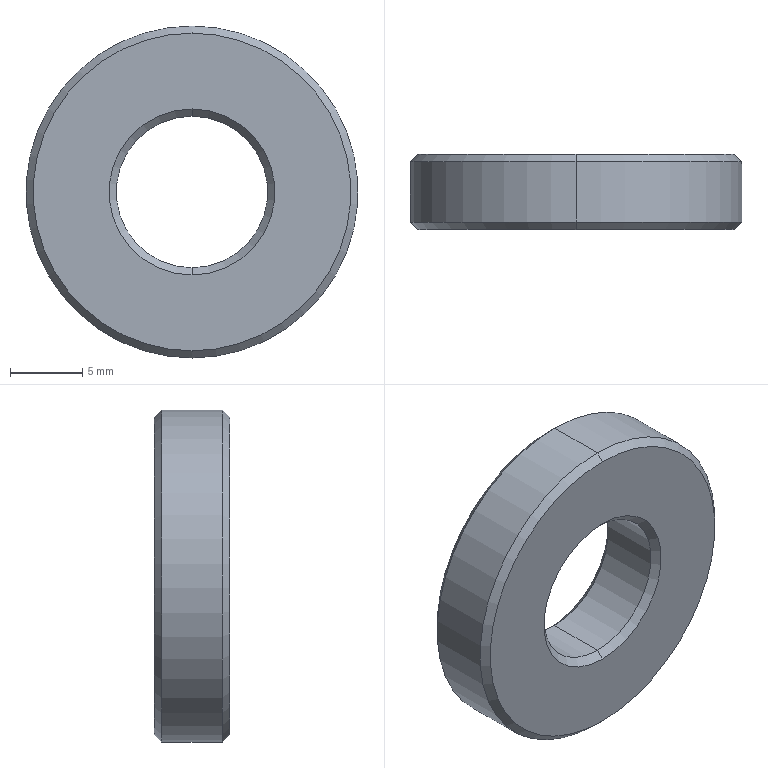Part | STEP file | ND25021-01-JDKM-06-SL | 1 solid | 14 faces | box 23 x 5.2 x 23 mm | volume 1684 mm3 | cone 8 | cylinder 4 | plane 2 | commonest cylinder face diameters 10.5 x2 23 x2
STEP:
#1=CARTESIAN_POINT('',(0.,0.,0.));
#2=DIRECTION('',(0.,0.,1.));
#3=DIRECTION('',(1.,0.,0.));
#4=AXIS2_PLACEMENT_3D('',#1,#2,#3);
#5=CARTESIAN_POINT('',(0.,4.7,5.25));
#6=VERTEX_POINT('',#5);
#7=CARTESIAN_POINT('',(0.,5.2,5.75));
#8=VERTEX_POINT('',#7);
#9=CARTESIAN_POINT('',(0.,4.7,5.25));
#10=DIRECTION('',(0.,0.7071,0.7071));
#11=VECTOR('',#10,1.);
#12=LINE('',#9,#11);
#13=CARTESIAN_POINT('',(0.,4.7,0.));
#14=DIRECTION('',(0.,1.,0.));
#15=DIRECTION('',(0.,0.,1.));
#16=AXIS2_PLACEMENT_3D('',#13,#14,#15);
#17=CONICAL_SURFACE('',#16,5.25,0.7854);
#18=CARTESIAN_POINT('',(6.283,0.));
#19=DIRECTION('',(0.,1.));
#20=VECTOR('',#19,1.);
#21=LINE('',#18,#20);
#22=(GEOMETRIC_REPRESENTATION_CONTEXT(2)PARAMETRIC_REPRESENTATION_CONTEXT()REPRESENTATION_CONTEXT('',''));
#23=DEFINITIONAL_REPRESENTATION('',(#21),#22);
#24=PCURVE('',#17,#23);
#25=CARTESIAN_POINT('',(0.,4.7,0.));
#26=DIRECTION('',(0.,1.,0.));
#27=DIRECTION('',(0.,0.,1.));
#28=AXIS2_PLACEMENT_3D('',#25,#26,#27);
#29=CONICAL_SURFACE('',#28,5.25,0.7854);
#30=CARTESIAN_POINT('',(0.,0.));
#31=DIRECTION('',(0.,1.));
#32=VECTOR('',#31,1.);
#33=LINE('',#30,#32);
#34=(GEOMETRIC_REPRESENTATION_CONTEXT(2)PARAMETRIC_REPRESENTATION_CONTEXT()REPRESENTATION_CONTEXT('',''));
#35=DEFINITIONAL_REPRESENTATION('',(#33),#34);
#36=PCURVE('',#29,#35);
#37=SURFACE_CURVE('',#12,(#24,#36),.PCURVE_S1.);
#38=EDGE_CURVE('',#6,#8,#37,.T.);
#39=ORIENTED_EDGE('',*,*,#38,.T.);
#40=CARTESIAN_POINT('',(0.,5.2,-5.75));
#41=VERTEX_POINT('',#40);
#42=CARTESIAN_POINT('',(0.,5.2,0.));
#43=DIRECTION('',(0.,-1.,0.));
#44=DIRECTION('',(0.,0.,1.));
#45=AXIS2_PLACEMENT_3D('',#42,#43,#44);
#46=CIRCLE('',#45,5.75);
#47=CARTESIAN_POINT('',(6.283,0.5));
#48=DIRECTION('',(-1.,0.));
#49=VECTOR('',#48,1.);
#50=LINE('',#47,#49);
#51=(GEOMETRIC_REPRESENTATION_CONTEXT(2)PARAMETRIC_REPRESENTATION_CONTEXT()REPRESENTATION_CONTEXT('',''));
#52=DEFINITIONAL_REPRESENTATION('',(#50),#51);
#53=PCURVE('',#17,#52);
#54=CARTESIAN_POINT('',(0.,5.2,0.));
#55=DIRECTION('',(0.,1.,0.));
#56=DIRECTION('',(0.,0.,1.));
#57=AXIS2_PLACEMENT_3D('',#54,#55,#56);
#58=PLANE('',#57);
#59=CARTESIAN_POINT('',(5.75,0.));
#60=CARTESIAN_POINT('',(5.75,-9.959));
#61=CARTESIAN_POINT('',(-2.875,-4.98));
#62=CARTESIAN_POINT('',(-11.5,0.));
#63=CARTESIAN_POINT('',(-2.875,4.98));
#64=CARTESIAN_POINT('',(5.75,9.959));
#65=CARTESIAN_POINT('',(5.75,0.));
#66=(BOUNDED_CURVE()B_SPLINE_CURVE(2,(#59,#60,#61,#62,#63,#64,#65),.UNSPECIFIED.,.T.,.F.)B_SPLINE_CURVE_WITH_KNOTS((1,2,2,2,2,1),(-2.094,0.,2.094,4.189,6.283,8.378),.UNSPECIFIED.)CURVE()GEOMETRIC_REPRESENTATION_ITEM()RATIONAL_B_SPLINE_CURVE((1.,0.5,1.,0.5,1.,0.5,1.))REPRESENTATION_ITEM(''));
#67=(GEOMETRIC_REPRESENTATION_CONTEXT(2)PARAMETRIC_REPRESENTATION_CONTEXT()REPRESENTATION_CONTEXT('',''));
#68=DEFINITIONAL_REPRESENTATION('',(#66),#67);
#69=PCURVE('',#58,#68);
#70=SURFACE_CURVE('',#46,(#53,#69),.PCURVE_S1.);
#71=EDGE_CURVE('',#8,#41,#70,.T.);
#72=ORIENTED_EDGE('',*,*,#71,.T.);
#73=CARTESIAN_POINT('',(0.,4.7,-5.25));
#74=VERTEX_POINT('',#73);
#75=CARTESIAN_POINT('',(0.,4.7,-5.25));
#76=DIRECTION('',(0.,0.7071,-0.7071));
#77=VECTOR('',#76,1.);
#78=LINE('',#75,#77);
#79=CARTESIAN_POINT('',(3.142,0.));
#80=DIRECTION('',(0.,1.));
#81=VECTOR('',#80,1.);
#82=LINE('',#79,#81);
#83=(GEOMETRIC_REPRESENTATION_CONTEXT(2)PARAMETRIC_REPRESENTATION_CONTEXT()REPRESENTATION_CONTEXT('',''));
#84=DEFINITIONAL_REPRESENTATION('',(#82),#83);
#85=PCURVE('',#17,#84);
#86=CARTESIAN_POINT('',(3.142,0.));
#87=DIRECTION('',(0.,1.));
#88=VECTOR('',#87,1.);
#89=LINE('',#86,#88);
#90=(GEOMETRIC_REPRESENTATION_CONTEXT(2)PARAMETRIC_REPRESENTATION_CONTEXT()REPRESENTATION_CONTEXT('',''));
#91=DEFINITIONAL_REPRESENTATION('',(#89),#90);
#92=PCURVE('',#29,#91);
#93=SURFACE_CURVE('',#78,(#85,#92),.PCURVE_S1.);
#94=EDGE_CURVE('',#74,#41,#93,.T.);
#95=ORIENTED_EDGE('',*,*,#94,.F.);
#96=CARTESIAN_POINT('',(0.,4.7,0.));
#97=DIRECTION('',(0.,1.,0.));
#98=DIRECTION('',(0.,0.,1.));
#99=AXIS2_PLACEMENT_3D('',#96,#97,#98);
#100=CIRCLE('',#99,5.25);
#101=CARTESIAN_POINT('',(0.,0.));
#102=DIRECTION('',(1.,0.));
#103=VECTOR('',#102,1.);
#104=LINE('',#101,#103);
#105=(GEOMETRIC_REPRESENTATION_CONTEXT(2)PARAMETRIC_REPRESENTATION_CONTEXT()REPRESENTATION_CONTEXT('',''));
#106=DEFINITIONAL_REPRESENTATION('',(#104),#105);
#107=PCURVE('',#17,#106);
#108=CARTESIAN_POINT('',(0.,5.2,0.));
#109=DIRECTION('',(0.,-1.,0.));
#110=DIRECTION('',(0.,0.,-1.));
#111=AXIS2_PLACEMENT_3D('',#108,#109,#110);
#112=CYLINDRICAL_SURFACE('',#111,5.25);
#113=CARTESIAN_POINT('',(9.425,0.5));
#114=DIRECTION('',(-1.,0.));
#115=VECTOR('',#114,1.);
#116=LINE('',#113,#115);
#117=(GEOMETRIC_REPRESENTATION_CONTEXT(2)PARAMETRIC_REPRESENTATION_CONTEXT()REPRESENTATION_CONTEXT('',''));
#118=DEFINITIONAL_REPRESENTATION('',(#116),#117);
#119=PCURVE('',#112,#118);
#120=SURFACE_CURVE('',#100,(#107,#119),.PCURVE_S1.);
#121=EDGE_CURVE('',#74,#6,#120,.T.);
#122=ORIENTED_EDGE('',*,*,#121,.T.);
#123=EDGE_LOOP('',(#39,#72,#95,#122));
#124=FACE_BOUND('',#123,.F.);
#125=ADVANCED_FACE('',(#124),#17,.F.);
#126=CARTESIAN_POINT('',(0.,0.5,-5.25));
#127=VERTEX_POINT('',#126);
#128=CARTESIAN_POINT('',(0.,0.,-5.75));
#129=VERTEX_POINT('',#128);
#130=CARTESIAN_POINT('',(0.,0.,-5.75));
#131=DIRECTION('',(0.,-0.7071,-0.7071));
#132=VECTOR('',#131,1.);
#133=LINE('',#130,#132);
#134=CARTESIAN_POINT('',(0.,0.,0.));
#135=DIRECTION('',(0.,-1.,0.));
#136=DIRECTION('',(0.,0.,-1.));
#137=AXIS2_PLACEMENT_3D('',#134,#135,#136);
#138=CONICAL_SURFACE('',#137,5.75,0.7854);
#139=CARTESIAN_POINT('',(6.283,0.));
#140=DIRECTION('',(0.,1.));
#141=VECTOR('',#140,1.);
#142=LINE('',#139,#141);
#143=(GEOMETRIC_REPRESENTATION_CONTEXT(2)PARAMETRIC_REPRESENTATION_CONTEXT()REPRESENTATION_CONTEXT('',''));
#144=DEFINITIONAL_REPRESENTATION('',(#142),#143);
#145=PCURVE('',#138,#144);
#146=CARTESIAN_POINT('',(0.,0.,0.));
#147=DIRECTION('',(0.,-1.,0.));
#148=DIRECTION('',(0.,0.,-1.));
#149=AXIS2_PLACEMENT_3D('',#146,#147,#148);
#150=CONICAL_SURFACE('',#149,5.75,0.7854);
#151=CARTESIAN_POINT('',(0.,0.));
#152=DIRECTION('',(0.,1.));
#153=VECTOR('',#152,1.);
#154=LINE('',#151,#153);
#155=(GEOMETRIC_REPRESENTATION_CONTEXT(2)PARAMETRIC_REPRESENTATION_CONTEXT()REPRESENTATION_CONTEXT('',''));
#156=DEFINITIONAL_REPRESENTATION('',(#154),#155);
#157=PCURVE('',#150,#156);
#158=SURFACE_CURVE('',#133,(#145,#157),.PCURVE_S1.);
#159=EDGE_CURVE('',#127,#129,#158,.T.);
#160=ORIENTED_EDGE('',*,*,#159,.T.);
#161=CARTESIAN_POINT('',(0.,0.,5.75));
#162=VERTEX_POINT('',#161);
#163=CARTESIAN_POINT('',(0.,0.,0.));
#164=DIRECTION('',(0.,1.,0.));
#165=DIRECTION('',(0.,0.,1.));
#166=AXIS2_PLACEMENT_3D('',#163,#164,#165);
#167=CIRCLE('',#166,5.75);
#168=CARTESIAN_POINT('',(9.425,0.));
#169=DIRECTION('',(-1.,0.));
#170=VECTOR('',#169,1.);
#171=LINE('',#168,#170);
#172=(GEOMETRIC_REPRESENTATION_CONTEXT(2)PARAMETRIC_REPRESENTATION_CONTEXT()REPRESENTATION_CONTEXT('',''));
#173=DEFINITIONAL_REPRESENTATION('',(#171),#172);
#174=PCURVE('',#138,#173);
#175=CARTESIAN_POINT('',(0.,0.,0.));
#176=DIRECTION('',(0.,1.,0.));
#177=DIRECTION('',(0.,0.,1.));
#178=AXIS2_PLACEMENT_3D('',#175,#176,#177);
#179=PLANE('',#178);
#180=CARTESIAN_POINT('',(0.,0.));
#181=DIRECTION('',(1.,0.));
#182=AXIS2_PLACEMENT_2D('',#180,#181);
#183=CIRCLE('',#182,5.75);
#184=(GEOMETRIC_REPRESENTATION_CONTEXT(2)PARAMETRIC_REPRESENTATION_CONTEXT()REPRESENTATION_CONTEXT('',''));
#185=DEFINITIONAL_REPRESENTATION('',(#183),#184);
#186=PCURVE('',#179,#185);
#187=SURFACE_CURVE('',#167,(#174,#186),.PCURVE_S1.);
#188=EDGE_CURVE('',#129,#162,#187,.T.);
#189=ORIENTED_EDGE('',*,*,#188,.T.);
#190=CARTESIAN_POINT('',(0.,0.5,5.25));
#191=VERTEX_POINT('',#190);
#192=CARTESIAN_POINT('',(0.,0.,5.75));
#193=DIRECTION('',(0.,-0.7071,0.7071));
#194=VECTOR('',#193,1.);
#195=LINE('',#192,#194);
#196=CARTESIAN_POINT('',(3.142,0.));
#197=DIRECTION('',(0.,1.));
#198=VECTOR('',#197,1.);
#199=LINE('',#196,#198);
#200=(GEOMETRIC_REPRESENTATION_CONTEXT(2)PARAMETRIC_REPRESENTATION_CONTEXT()REPRESENTATION_CONTEXT('',''));
#201=DEFINITIONAL_REPRESENTATION('',(#199),#200);
#202=PCURVE('',#138,#201);
#203=CARTESIAN_POINT('',(3.142,0.));
#204=DIRECTION('',(0.,1.));
#205=VECTOR('',#204,1.);
#206=LINE('',#203,#205);
#207=(GEOMETRIC_REPRESENTATION_CONTEXT(2)PARAMETRIC_REPRESENTATION_CONTEXT()REPRESENTATION_CONTEXT('',''));
#208=DEFINITIONAL_REPRESENTATION('',(#206),#207);
#209=PCURVE('',#150,#208);
#210=SURFACE_CURVE('',#195,(#202,#209),.PCURVE_S1.);
#211=EDGE_CURVE('',#191,#162,#210,.T.);
#212=ORIENTED_EDGE('',*,*,#211,.F.);
#213=CARTESIAN_POINT('',(0.,0.5,0.));
#214=DIRECTION('',(0.,-1.,0.));
#215=DIRECTION('',(0.,0.,1.));
#216=AXIS2_PLACEMENT_3D('',#213,#214,#215);
#217=CIRCLE('',#216,5.25);
#218=CARTESIAN_POINT('',(3.142,-0.5));
#219=DIRECTION('',(1.,0.));
#220=VECTOR('',#219,1.);
#221=LINE('',#218,#220);
#222=(GEOMETRIC_REPRESENTATION_CONTEXT(2)PARAMETRIC_REPRESENTATION_CONTEXT()REPRESENTATION_CONTEXT('',''));
#223=DEFINITIONAL_REPRESENTATION('',(#221),#222);
#224=PCURVE('',#138,#223);
#225=CARTESIAN_POINT('',(3.142,4.7));
#226=DIRECTION('',(1.,0.));
#227=VECTOR('',#226,1.);
#228=LINE('',#225,#227);
#229=(GEOMETRIC_REPRESENTATION_CONTEXT(2)PARAMETRIC_REPRESENTATION_CONTEXT()REPRESENTATION_CONTEXT('',''));
#230=DEFINITIONAL_REPRESENTATION('',(#228),#229);
#231=PCURVE('',#112,#230);
#232=SURFACE_CURVE('',#217,(#224,#231),.PCURVE_S1.);
#233=EDGE_CURVE('',#191,#127,#232,.T.);
#234=ORIENTED_EDGE('',*,*,#233,.T.);
#235=EDGE_LOOP('',(#160,#189,#212,#234));
#236=FACE_BOUND('',#235,.F.);
#237=ADVANCED_FACE('',(#236),#138,.F.);
#238=CARTESIAN_POINT('',(0.,5.2,11.));
#239=VERTEX_POINT('',#238);
#240=CARTESIAN_POINT('',(0.,5.2,-11.));
#241=VERTEX_POINT('',#240);
#242=CARTESIAN_POINT('',(0.,5.2,0.));
#243=DIRECTION('',(0.,1.,0.));
#244=DIRECTION('',(0.,0.,1.));
#245=AXIS2_PLACEMENT_3D('',#242,#243,#244);
#246=CIRCLE('',#245,11.);
#247=CARTESIAN_POINT('',(0.,5.2,0.));
#248=DIRECTION('',(0.,-1.,0.));
#249=DIRECTION('',(0.,0.,-1.));
#250=AXIS2_PLACEMENT_3D('',#247,#248,#249);
#251=CONICAL_SURFACE('',#250,11.,0.7854);
#252=CARTESIAN_POINT('',(3.142,0.));
#253=DIRECTION('',(-1.,0.));
#254=VECTOR('',#253,1.);
#255=LINE('',#252,#254);
#256=(GEOMETRIC_REPRESENTATION_CONTEXT(2)PARAMETRIC_REPRESENTATION_CONTEXT()REPRESENTATION_CONTEXT('',''));
#257=DEFINITIONAL_REPRESENTATION('',(#255),#256);
#258=PCURVE('',#251,#257);
#259=CARTESIAN_POINT('',(0.,0.));
#260=DIRECTION('',(1.,0.));
#261=AXIS2_PLACEMENT_2D('',#259,#260);
#262=CIRCLE('',#261,11.);
#263=(GEOMETRIC_REPRESENTATION_CONTEXT(2)PARAMETRIC_REPRESENTATION_CONTEXT()REPRESENTATION_CONTEXT('',''));
#264=DEFINITIONAL_REPRESENTATION('',(#262),#263);
#265=PCURVE('',#58,#264);
#266=SURFACE_CURVE('',#246,(#258,#265),.PCURVE_S1.);
#267=EDGE_CURVE('',#239,#241,#266,.T.);
#268=ORIENTED_EDGE('',*,*,#267,.F.);
#269=CARTESIAN_POINT('',(0.,4.7,11.5));
#270=VERTEX_POINT('',#269);
#271=CARTESIAN_POINT('',(0.,5.2,11.));
#272=DIRECTION('',(0.,-0.7071,0.7071));
#273=VECTOR('',#272,1.);
#274=LINE('',#271,#273);
#275=CARTESIAN_POINT('',(3.142,0.));
#276=DIRECTION('',(0.,1.));
#277=VECTOR('',#276,1.);
#278=LINE('',#275,#277);
#279=(GEOMETRIC_REPRESENTATION_CONTEXT(2)PARAMETRIC_REPRESENTATION_CONTEXT()REPRESENTATION_CONTEXT('',''));
#280=DEFINITIONAL_REPRESENTATION('',(#278),#279);
#281=PCURVE('',#251,#280);
#282=CARTESIAN_POINT('',(0.,5.2,0.));
#283=DIRECTION('',(0.,-1.,0.));
#284=DIRECTION('',(0.,0.,-1.));
#285=AXIS2_PLACEMENT_3D('',#282,#283,#284);
#286=CONICAL_SURFACE('',#285,11.,0.7854);
#287=CARTESIAN_POINT('',(3.142,0.));
#288=DIRECTION('',(0.,1.));
#289=VECTOR('',#288,1.);
#290=LINE('',#287,#289);
#291=(GEOMETRIC_REPRESENTATION_CONTEXT(2)PARAMETRIC_REPRESENTATION_CONTEXT()REPRESENTATION_CONTEXT('',''));
#292=DEFINITIONAL_REPRESENTATION('',(#290),#291);
#293=PCURVE('',#286,#292);
#294=SURFACE_CURVE('',#274,(#281,#293),.PCURVE_S1.);
#295=EDGE_CURVE('',#239,#270,#294,.T.);
#296=ORIENTED_EDGE('',*,*,#295,.T.);
#297=CARTESIAN_POINT('',(0.,4.7,-11.5));
#298=VERTEX_POINT('',#297);
#299=CARTESIAN_POINT('',(0.,4.7,0.));
#300=DIRECTION('',(0.,-1.,0.));
#301=DIRECTION('',(0.,0.,1.));
#302=AXIS2_PLACEMENT_3D('',#299,#300,#301);
#303=CIRCLE('',#302,11.5);
#304=CARTESIAN_POINT('',(-3.142,0.5));
#305=DIRECTION('',(1.,0.));
#306=VECTOR('',#305,1.);
#307=LINE('',#304,#306);
#308=(GEOMETRIC_REPRESENTATION_CONTEXT(2)PARAMETRIC_REPRESENTATION_CONTEXT()REPRESENTATION_CONTEXT('',''));
#309=DEFINITIONAL_REPRESENTATION('',(#307),#308);
#310=PCURVE('',#251,#309);
#311=CARTESIAN_POINT('',(0.,5.2,0.));
#312=DIRECTION('',(0.,-1.,0.));
#313=DIRECTION('',(0.,0.,-1.));
#314=AXIS2_PLACEMENT_3D('',#311,#312,#313);
#315=CYLINDRICAL_SURFACE('',#314,11.5);
#316=CARTESIAN_POINT('',(-3.142,0.5));
#317=DIRECTION('',(1.,0.));
#318=VECTOR('',#317,1.);
#319=LINE('',#316,#318);
#320=(GEOMETRIC_REPRESENTATION_CONTEXT(2)PARAMETRIC_REPRESENTATION_CONTEXT()REPRESENTATION_CONTEXT('',''));
#321=DEFINITIONAL_REPRESENTATION('',(#319),#320);
#322=PCURVE('',#315,#321);
#323=SURFACE_CURVE('',#303,(#310,#322),.PCURVE_S1.);
#324=EDGE_CURVE('',#298,#270,#323,.T.);
#325=ORIENTED_EDGE('',*,*,#324,.F.);
#326=CARTESIAN_POINT('',(0.,5.2,-11.));
#327=DIRECTION('',(0.,-0.7071,-0.7071));
#328=VECTOR('',#327,1.);
#329=LINE('',#326,#328);
#330=CARTESIAN_POINT('',(0.,0.));
#331=DIRECTION('',(0.,1.));
#332=VECTOR('',#331,1.);
#333=LINE('',#330,#332);
#334=(GEOMETRIC_REPRESENTATION_CONTEXT(2)PARAMETRIC_REPRESENTATION_CONTEXT()REPRESENTATION_CONTEXT('',''));
#335=DEFINITIONAL_REPRESENTATION('',(#333),#334);
#336=PCURVE('',#251,#335);
#337=CARTESIAN_POINT('',(6.283,0.));
#338=DIRECTION('',(0.,1.));
#339=VECTOR('',#338,1.);
#340=LINE('',#337,#339);
#341=(GEOMETRIC_REPRESENTATION_CONTEXT(2)PARAMETRIC_REPRESENTATION_CONTEXT()REPRESENTATION_CONTEXT('',''));
#342=DEFINITIONAL_REPRESENTATION('',(#340),#341);
#343=PCURVE('',#286,#342);
#344=SURFACE_CURVE('',#329,(#336,#343),.PCURVE_S1.);
#345=EDGE_CURVE('',#241,#298,#344,.T.);
#346=ORIENTED_EDGE('',*,*,#345,.F.);
#347=EDGE_LOOP('',(#268,#296,#325,#346));
#348=FACE_BOUND('',#347,.T.);
#349=ADVANCED_FACE('',(#348),#251,.T.);
#350=CARTESIAN_POINT('',(0.,0.,-11.));
#351=VERTEX_POINT('',#350);
#352=CARTESIAN_POINT('',(0.,0.,11.));
#353=VERTEX_POINT('',#352);
#354=CARTESIAN_POINT('',(0.,0.,0.));
#355=DIRECTION('',(0.,-1.,0.));
#356=DIRECTION('',(0.,0.,1.));
#357=AXIS2_PLACEMENT_3D('',#354,#355,#356);
#358=CIRCLE('',#357,11.);
#359=CARTESIAN_POINT('',(0.,0.5,0.));
#360=DIRECTION('',(0.,1.,0.));
#361=DIRECTION('',(0.,0.,1.));
#362=AXIS2_PLACEMENT_3D('',#359,#360,#361);
#363=CONICAL_SURFACE('',#362,11.5,0.7854);
#364=CARTESIAN_POINT('',(6.283,-0.5));
#365=DIRECTION('',(-1.,0.));
#366=VECTOR('',#365,1.);
#367=LINE('',#364,#366);
#368=(GEOMETRIC_REPRESENTATION_CONTEXT(2)PARAMETRIC_REPRESENTATION_CONTEXT()REPRESENTATION_CONTEXT('',''));
#369=DEFINITIONAL_REPRESENTATION('',(#367),#368);
#370=PCURVE('',#363,#369);
#371=CARTESIAN_POINT('',(11.,0.));
#372=CARTESIAN_POINT('',(11.,-19.053));
#373=CARTESIAN_POINT('',(-5.5,-9.526));
#374=CARTESIAN_POINT('',(-22.,0.));
#375=CARTESIAN_POINT('',(-5.5,9.526));
#376=CARTESIAN_POINT('',(11.,19.053));
#377=CARTESIAN_POINT('',(11.,0.));
#378=(BOUNDED_CURVE()B_SPLINE_CURVE(2,(#371,#372,#373,#374,#375,#376,#377),.UNSPECIFIED.,.T.,.F.)B_SPLINE_CURVE_WITH_KNOTS((1,2,2,2,2,1),(-2.094,0.,2.094,4.189,6.283,8.378),.UNSPECIFIED.)CURVE()GEOMETRIC_REPRESENTATION_ITEM()RATIONAL_B_SPLINE_CURVE((1.,0.5,1.,0.5,1.,0.5,1.))REPRESENTATION_ITEM(''));
#379=(GEOMETRIC_REPRESENTATION_CONTEXT(2)PARAMETRIC_REPRESENTATION_CONTEXT()REPRESENTATION_CONTEXT('',''));
#380=DEFINITIONAL_REPRESENTATION('',(#378),#379);
#381=PCURVE('',#179,#380);
#382=SURFACE_CURVE('',#358,(#370,#381),.PCURVE_S1.);
#383=EDGE_CURVE('',#351,#353,#382,.T.);
#384=ORIENTED_EDGE('',*,*,#383,.F.);
#385=CARTESIAN_POINT('',(0.,0.5,-11.5));
#386=VERTEX_POINT('',#385);
#387=CARTESIAN_POINT('',(0.,0.5,-11.5));
#388=DIRECTION('',(0.,0.7071,-0.7071));
#389=VECTOR('',#388,1.);
#390=LINE('',#387,#389);
#391=CARTESIAN_POINT('',(3.142,0.));
#392=DIRECTION('',(0.,1.));
#393=VECTOR('',#392,1.);
#394=LINE('',#391,#393);
#395=(GEOMETRIC_REPRESENTATION_CONTEXT(2)PARAMETRIC_REPRESENTATION_CONTEXT()REPRESENTATION_CONTEXT('',''));
#396=DEFINITIONAL_REPRESENTATION('',(#394),#395);
#397=PCURVE('',#363,#396);
#398=CARTESIAN_POINT('',(0.,0.5,0.));
#399=DIRECTION('',(0.,1.,0.));
#400=DIRECTION('',(0.,0.,1.));
#401=AXIS2_PLACEMENT_3D('',#398,#399,#400);
#402=CONICAL_SURFACE('',#401,11.5,0.7854);
#403=CARTESIAN_POINT('',(3.142,0.));
#404=DIRECTION('',(0.,1.));
#405=VECTOR('',#404,1.);
#406=LINE('',#403,#405);
#407=(GEOMETRIC_REPRESENTATION_CONTEXT(2)PARAMETRIC_REPRESENTATION_CONTEXT()REPRESENTATION_CONTEXT('',''));
#408=DEFINITIONAL_REPRESENTATION('',(#406),#407);
#409=PCURVE('',#402,#408);
#410=SURFACE_CURVE('',#390,(#397,#409),.PCURVE_S1.);
#411=EDGE_CURVE('',#351,#386,#410,.T.);
#412=ORIENTED_EDGE('',*,*,#411,.T.);
#413=CARTESIAN_POINT('',(0.,0.5,11.5));
#414=VERTEX_POINT('',#413);
#415=CARTESIAN_POINT('',(0.,0.5,0.));
#416=DIRECTION('',(0.,1.,0.));
#417=DIRECTION('',(0.,0.,1.));
#418=AXIS2_PLACEMENT_3D('',#415,#416,#417);
#419=CIRCLE('',#418,11.5);
#420=CARTESIAN_POINT('',(0.,0.));
#421=DIRECTION('',(1.,0.));
#422=VECTOR('',#421,1.);
#423=LINE('',#420,#422);
#424=(GEOMETRIC_REPRESENTATION_CONTEXT(2)PARAMETRIC_REPRESENTATION_CONTEXT()REPRESENTATION_CONTEXT('',''));
#425=DEFINITIONAL_REPRESENTATION('',(#423),#424);
#426=PCURVE('',#363,#425);
#427=CARTESIAN_POINT('',(3.142,4.7));
#428=DIRECTION('',(-1.,0.));
#429=VECTOR('',#428,1.);
#430=LINE('',#427,#429);
#431=(GEOMETRIC_REPRESENTATION_CONTEXT(2)PARAMETRIC_REPRESENTATION_CONTEXT()REPRESENTATION_CONTEXT('',''));
#432=DEFINITIONAL_REPRESENTATION('',(#430),#431);
#433=PCURVE('',#315,#432);
#434=SURFACE_CURVE('',#419,(#426,#433),.PCURVE_S1.);
#435=EDGE_CURVE('',#414,#386,#434,.T.);
#436=ORIENTED_EDGE('',*,*,#435,.F.);
#437=CARTESIAN_POINT('',(0.,0.5,11.5));
#438=DIRECTION('',(0.,0.7071,0.7071));
#439=VECTOR('',#438,1.);
#440=LINE('',#437,#439);
#441=CARTESIAN_POINT('',(0.,0.));
#442=DIRECTION('',(0.,1.));
#443=VECTOR('',#442,1.);
#444=LINE('',#441,#443);
#445=(GEOMETRIC_REPRESENTATION_CONTEXT(2)PARAMETRIC_REPRESENTATION_CONTEXT()REPRESENTATION_CONTEXT('',''));
#446=DEFINITIONAL_REPRESENTATION('',(#444),#445);
#447=PCURVE('',#363,#446);
#448=CARTESIAN_POINT('',(6.283,0.));
#449=DIRECTION('',(0.,1.));
#450=VECTOR('',#449,1.);
#451=LINE('',#448,#450);
#452=(GEOMETRIC_REPRESENTATION_CONTEXT(2)PARAMETRIC_REPRESENTATION_CONTEXT()REPRESENTATION_CONTEXT('',''));
#453=DEFINITIONAL_REPRESENTATION('',(#451),#452);
#454=PCURVE('',#402,#453);
#455=SURFACE_CURVE('',#440,(#447,#454),.PCURVE_S1.);
#456=EDGE_CURVE('',#353,#414,#455,.T.);
#457=ORIENTED_EDGE('',*,*,#456,.F.);
#458=EDGE_LOOP('',(#384,#412,#436,#457));
#459=FACE_BOUND('',#458,.T.);
#460=ADVANCED_FACE('',(#459),#363,.T.);
#461=CARTESIAN_POINT('',(0.,5.2,-5.25));
#462=DIRECTION('',(0.,-1.,0.));
#463=VECTOR('',#462,1.);
#464=LINE('',#461,#463);
#465=CARTESIAN_POINT('',(6.283,0.));
#466=DIRECTION('',(0.,1.));
#467=VECTOR('',#466,1.);
#468=LINE('',#465,#467);
#469=(GEOMETRIC_REPRESENTATION_CONTEXT(2)PARAMETRIC_REPRESENTATION_CONTEXT()REPRESENTATION_CONTEXT('',''));
#470=DEFINITIONAL_REPRESENTATION('',(#468),#469);
#471=PCURVE('',#112,#470);
#472=CARTESIAN_POINT('',(0.,5.2,0.));
#473=DIRECTION('',(0.,-1.,0.));
#474=DIRECTION('',(0.,0.,-1.));
#475=AXIS2_PLACEMENT_3D('',#472,#473,#474);
#476=CYLINDRICAL_SURFACE('',#475,5.25);
#477=CARTESIAN_POINT('',(0.,0.));
#478=DIRECTION('',(0.,1.));
#479=VECTOR('',#478,1.);
#480=LINE('',#477,#479);
#481=(GEOMETRIC_REPRESENTATION_CONTEXT(2)PARAMETRIC_REPRESENTATION_CONTEXT()REPRESENTATION_CONTEXT('',''));
#482=DEFINITIONAL_REPRESENTATION('',(#480),#481);
#483=PCURVE('',#476,#482);
#484=SURFACE_CURVE('',#464,(#471,#483),.PCURVE_S1.);
#485=EDGE_CURVE('',#74,#127,#484,.T.);
#486=ORIENTED_EDGE('',*,*,#485,.T.);
#487=ORIENTED_EDGE('',*,*,#233,.F.);
#488=CARTESIAN_POINT('',(0.,5.2,5.25));
#489=DIRECTION('',(0.,-1.,0.));
#490=VECTOR('',#489,1.);
#491=LINE('',#488,#490);
#492=CARTESIAN_POINT('',(3.142,0.));
#493=DIRECTION('',(0.,1.));
#494=VECTOR('',#493,1.);
#495=LINE('',#492,#494);
#496=(GEOMETRIC_REPRESENTATION_CONTEXT(2)PARAMETRIC_REPRESENTATION_CONTEXT()REPRESENTATION_CONTEXT('',''));
#497=DEFINITIONAL_REPRESENTATION('',(#495),#496);
#498=PCURVE('',#112,#497);
#499=CARTESIAN_POINT('',(3.142,0.));
#500=DIRECTION('',(0.,1.));
#501=VECTOR('',#500,1.);
#502=LINE('',#499,#501);
#503=(GEOMETRIC_REPRESENTATION_CONTEXT(2)PARAMETRIC_REPRESENTATION_CONTEXT()REPRESENTATION_CONTEXT('',''));
#504=DEFINITIONAL_REPRESENTATION('',(#502),#503);
#505=PCURVE('',#476,#504);
#506=SURFACE_CURVE('',#491,(#498,#505),.PCURVE_S1.);
#507=EDGE_CURVE('',#6,#191,#506,.T.);
#508=ORIENTED_EDGE('',*,*,#507,.F.);
#509=ORIENTED_EDGE('',*,*,#121,.F.);
#510=EDGE_LOOP('',(#486,#487,#508,#509));
#511=FACE_BOUND('',#510,.F.);
#512=ADVANCED_FACE('',(#511),#112,.F.);
#513=ORIENTED_EDGE('',*,*,#324,.T.);
#514=CARTESIAN_POINT('',(0.,5.2,11.5));
#515=DIRECTION('',(0.,-1.,0.));
#516=VECTOR('',#515,1.);
#517=LINE('',#514,#516);
#518=CARTESIAN_POINT('',(3.142,0.));
#519=DIRECTION('',(0.,1.));
#520=VECTOR('',#519,1.);
#521=LINE('',#518,#520);
#522=(GEOMETRIC_REPRESENTATION_CONTEXT(2)PARAMETRIC_REPRESENTATION_CONTEXT()REPRESENTATION_CONTEXT('',''));
#523=DEFINITIONAL_REPRESENTATION('',(#521),#522);
#524=PCURVE('',#315,#523);
#525=CARTESIAN_POINT('',(0.,5.2,0.));
#526=DIRECTION('',(0.,-1.,0.));
#527=DIRECTION('',(0.,0.,-1.));
#528=AXIS2_PLACEMENT_3D('',#525,#526,#527);
#529=CYLINDRICAL_SURFACE('',#528,11.5);
#530=CARTESIAN_POINT('',(3.142,0.));
#531=DIRECTION('',(0.,1.));
#532=VECTOR('',#531,1.);
#533=LINE('',#530,#532);
#534=(GEOMETRIC_REPRESENTATION_CONTEXT(2)PARAMETRIC_REPRESENTATION_CONTEXT()REPRESENTATION_CONTEXT('',''));
#535=DEFINITIONAL_REPRESENTATION('',(#533),#534);
#536=PCURVE('',#529,#535);
#537=SURFACE_CURVE('',#517,(#524,#536),.PCURVE_S1.);
#538=EDGE_CURVE('',#270,#414,#537,.T.);
#539=ORIENTED_EDGE('',*,*,#538,.T.);
#540=ORIENTED_EDGE('',*,*,#435,.T.);
#541=CARTESIAN_POINT('',(0.,5.2,-11.5));
#542=DIRECTION('',(0.,-1.,0.));
#543=VECTOR('',#542,1.);
#544=LINE('',#541,#543);
#545=CARTESIAN_POINT('',(0.,0.));
#546=DIRECTION('',(0.,1.));
#547=VECTOR('',#546,1.);
#548=LINE('',#545,#547);
#549=(GEOMETRIC_REPRESENTATION_CONTEXT(2)PARAMETRIC_REPRESENTATION_CONTEXT()REPRESENTATION_CONTEXT('',''));
#550=DEFINITIONAL_REPRESENTATION('',(#548),#549);
#551=PCURVE('',#315,#550);
#552=CARTESIAN_POINT('',(6.283,0.));
#553=DIRECTION('',(0.,1.));
#554=VECTOR('',#553,1.);
#555=LINE('',#552,#554);
#556=(GEOMETRIC_REPRESENTATION_CONTEXT(2)PARAMETRIC_REPRESENTATION_CONTEXT()REPRESENTATION_CONTEXT('',''));
#557=DEFINITIONAL_REPRESENTATION('',(#555),#556);
#558=PCURVE('',#529,#557);
#559=SURFACE_CURVE('',#544,(#551,#558),.PCURVE_S1.);
#560=EDGE_CURVE('',#298,#386,#559,.T.);
#561=ORIENTED_EDGE('',*,*,#560,.F.);
#562=EDGE_LOOP('',(#513,#539,#540,#561));
#563=FACE_BOUND('',#562,.T.);
#564=ADVANCED_FACE('',(#563),#315,.T.);
#565=CARTESIAN_POINT('',(0.,5.2,0.));
#566=DIRECTION('',(0.,1.,0.));
#567=DIRECTION('',(0.,0.,1.));
#568=AXIS2_PLACEMENT_3D('',#565,#566,#567);
#569=CIRCLE('',#568,11.);
#570=CARTESIAN_POINT('',(0.,0.));
#571=DIRECTION('',(1.,0.));
#572=AXIS2_PLACEMENT_2D('',#570,#571);
#573=CIRCLE('',#572,11.);
#574=(GEOMETRIC_REPRESENTATION_CONTEXT(2)PARAMETRIC_REPRESENTATION_CONTEXT()REPRESENTATION_CONTEXT('',''));
#575=DEFINITIONAL_REPRESENTATION('',(#573),#574);
#576=PCURVE('',#58,#575);
#577=CARTESIAN_POINT('',(9.425,0.));
#578=DIRECTION('',(-1.,0.));
#579=VECTOR('',#578,1.);
#580=LINE('',#577,#579);
#581=(GEOMETRIC_REPRESENTATION_CONTEXT(2)PARAMETRIC_REPRESENTATION_CONTEXT()REPRESENTATION_CONTEXT('',''));
#582=DEFINITIONAL_REPRESENTATION('',(#580),#581);
#583=PCURVE('',#286,#582);
#584=SURFACE_CURVE('',#569,(#576,#583),.PCURVE_S1.);
#585=EDGE_CURVE('',#241,#239,#584,.T.);
#586=ORIENTED_EDGE('',*,*,#585,.T.);
#587=ORIENTED_EDGE('',*,*,#267,.T.);
#588=EDGE_LOOP('',(#586,#587));
#589=FACE_BOUND('',#588,.T.);
#590=ORIENTED_EDGE('',*,*,#71,.T.);
#591=CARTESIAN_POINT('',(0.,5.2,0.));
#592=DIRECTION('',(0.,-1.,0.));
#593=DIRECTION('',(0.,0.,1.));
#594=AXIS2_PLACEMENT_3D('',#591,#592,#593);
#595=CIRCLE('',#594,5.75);
#596=CARTESIAN_POINT('',(5.75,0.));
#597=CARTESIAN_POINT('',(5.75,-9.959));
#598=CARTESIAN_POINT('',(-2.875,-4.98));
#599=CARTESIAN_POINT('',(-11.5,0.));
#600=CARTESIAN_POINT('',(-2.875,4.98));
#601=CARTESIAN_POINT('',(5.75,9.959));
#602=CARTESIAN_POINT('',(5.75,0.));
#603=(BOUNDED_CURVE()B_SPLINE_CURVE(2,(#596,#597,#598,#599,#600,#601,#602),.UNSPECIFIED.,.T.,.F.)B_SPLINE_CURVE_WITH_KNOTS((1,2,2,2,2,1),(-2.094,0.,2.094,4.189,6.283,8.378),.UNSPECIFIED.)CURVE()GEOMETRIC_REPRESENTATION_ITEM()RATIONAL_B_SPLINE_CURVE((1.,0.5,1.,0.5,1.,0.5,1.))REPRESENTATION_ITEM(''));
#604=(GEOMETRIC_REPRESENTATION_CONTEXT(2)PARAMETRIC_REPRESENTATION_CONTEXT()REPRESENTATION_CONTEXT('',''));
#605=DEFINITIONAL_REPRESENTATION('',(#603),#604);
#606=PCURVE('',#58,#605);
#607=CARTESIAN_POINT('',(6.283,0.5));
#608=DIRECTION('',(-1.,0.));
#609=VECTOR('',#608,1.);
#610=LINE('',#607,#609);
#611=(GEOMETRIC_REPRESENTATION_CONTEXT(2)PARAMETRIC_REPRESENTATION_CONTEXT()REPRESENTATION_CONTEXT('',''));
#612=DEFINITIONAL_REPRESENTATION('',(#610),#611);
#613=PCURVE('',#29,#612);
#614=SURFACE_CURVE('',#595,(#606,#613),.PCURVE_S1.);
#615=EDGE_CURVE('',#41,#8,#614,.T.);
#616=ORIENTED_EDGE('',*,*,#615,.T.);
#617=EDGE_LOOP('',(#590,#616));
#618=FACE_BOUND('',#617,.T.);
#619=ADVANCED_FACE('',(#589,#618),#58,.T.);
#620=CARTESIAN_POINT('',(0.,0.,0.));
#621=DIRECTION('',(0.,-1.,0.));
#622=DIRECTION('',(0.,0.,1.));
#623=AXIS2_PLACEMENT_3D('',#620,#621,#622);
#624=CIRCLE('',#623,11.);
#625=CARTESIAN_POINT('',(11.,0.));
#626=CARTESIAN_POINT('',(11.,-19.053));
#627=CARTESIAN_POINT('',(-5.5,-9.526));
#628=CARTESIAN_POINT('',(-22.,0.));
#629=CARTESIAN_POINT('',(-5.5,9.526));
#630=CARTESIAN_POINT('',(11.,19.053));
#631=CARTESIAN_POINT('',(11.,0.));
#632=(BOUNDED_CURVE()B_SPLINE_CURVE(2,(#625,#626,#627,#628,#629,#630,#631),.UNSPECIFIED.,.T.,.F.)B_SPLINE_CURVE_WITH_KNOTS((1,2,2,2,2,1),(-2.094,0.,2.094,4.189,6.283,8.378),.UNSPECIFIED.)CURVE()GEOMETRIC_REPRESENTATION_ITEM()RATIONAL_B_SPLINE_CURVE((1.,0.5,1.,0.5,1.,0.5,1.))REPRESENTATION_ITEM(''));
#633=(GEOMETRIC_REPRESENTATION_CONTEXT(2)PARAMETRIC_REPRESENTATION_CONTEXT()REPRESENTATION_CONTEXT('',''));
#634=DEFINITIONAL_REPRESENTATION('',(#632),#633);
#635=PCURVE('',#179,#634);
#636=CARTESIAN_POINT('',(6.283,-0.5));
#637=DIRECTION('',(-1.,0.));
#638=VECTOR('',#637,1.);
#639=LINE('',#636,#638);
#640=(GEOMETRIC_REPRESENTATION_CONTEXT(2)PARAMETRIC_REPRESENTATION_CONTEXT()REPRESENTATION_CONTEXT('',''));
#641=DEFINITIONAL_REPRESENTATION('',(#639),#640);
#642=PCURVE('',#402,#641);
#643=SURFACE_CURVE('',#624,(#635,#642),.PCURVE_S1.);
#644=EDGE_CURVE('',#353,#351,#643,.T.);
#645=ORIENTED_EDGE('',*,*,#644,.T.);
#646=ORIENTED_EDGE('',*,*,#383,.T.);
#647=EDGE_LOOP('',(#645,#646));
#648=FACE_BOUND('',#647,.T.);
#649=ORIENTED_EDGE('',*,*,#188,.T.);
#650=CARTESIAN_POINT('',(0.,0.,0.));
#651=DIRECTION('',(0.,1.,0.));
#652=DIRECTION('',(0.,0.,1.));
#653=AXIS2_PLACEMENT_3D('',#650,#651,#652);
#654=CIRCLE('',#653,5.75);
#655=CARTESIAN_POINT('',(0.,0.));
#656=DIRECTION('',(1.,0.));
#657=AXIS2_PLACEMENT_2D('',#655,#656);
#658=CIRCLE('',#657,5.75);
#659=(GEOMETRIC_REPRESENTATION_CONTEXT(2)PARAMETRIC_REPRESENTATION_CONTEXT()REPRESENTATION_CONTEXT('',''));
#660=DEFINITIONAL_REPRESENTATION('',(#658),#659);
#661=PCURVE('',#179,#660);
#662=CARTESIAN_POINT('',(3.142,0.));
#663=DIRECTION('',(-1.,0.));
#664=VECTOR('',#663,1.);
#665=LINE('',#662,#664);
#666=(GEOMETRIC_REPRESENTATION_CONTEXT(2)PARAMETRIC_REPRESENTATION_CONTEXT()REPRESENTATION_CONTEXT('',''));
#667=DEFINITIONAL_REPRESENTATION('',(#665),#666);
#668=PCURVE('',#150,#667);
#669=SURFACE_CURVE('',#654,(#661,#668),.PCURVE_S1.);
#670=EDGE_CURVE('',#162,#129,#669,.T.);
#671=ORIENTED_EDGE('',*,*,#670,.T.);
#672=EDGE_LOOP('',(#649,#671));
#673=FACE_BOUND('',#672,.T.);
#674=ADVANCED_FACE('',(#648,#673),#179,.F.);
#675=ORIENTED_EDGE('',*,*,#538,.F.);
#676=CARTESIAN_POINT('',(0.,4.7,0.));
#677=DIRECTION('',(0.,-1.,0.));
#678=DIRECTION('',(0.,0.,1.));
#679=AXIS2_PLACEMENT_3D('',#676,#677,#678);
#680=CIRCLE('',#679,11.5);
#681=CARTESIAN_POINT('',(3.142,0.5));
#682=DIRECTION('',(1.,0.));
#683=VECTOR('',#682,1.);
#684=LINE('',#681,#683);
#685=(GEOMETRIC_REPRESENTATION_CONTEXT(2)PARAMETRIC_REPRESENTATION_CONTEXT()REPRESENTATION_CONTEXT('',''));
#686=DEFINITIONAL_REPRESENTATION('',(#684),#685);
#687=PCURVE('',#529,#686);
#688=CARTESIAN_POINT('',(3.142,0.5));
#689=DIRECTION('',(1.,0.));
#690=VECTOR('',#689,1.);
#691=LINE('',#688,#690);
#692=(GEOMETRIC_REPRESENTATION_CONTEXT(2)PARAMETRIC_REPRESENTATION_CONTEXT()REPRESENTATION_CONTEXT('',''));
#693=DEFINITIONAL_REPRESENTATION('',(#691),#692);
#694=PCURVE('',#286,#693);
#695=SURFACE_CURVE('',#680,(#687,#694),.PCURVE_S1.);
#696=EDGE_CURVE('',#270,#298,#695,.T.);
#697=ORIENTED_EDGE('',*,*,#696,.T.);
#698=ORIENTED_EDGE('',*,*,#560,.T.);
#699=CARTESIAN_POINT('',(0.,0.5,0.));
#700=DIRECTION('',(0.,1.,0.));
#701=DIRECTION('',(0.,0.,1.));
#702=AXIS2_PLACEMENT_3D('',#699,#700,#701);
#703=CIRCLE('',#702,11.5);
#704=CARTESIAN_POINT('',(9.425,4.7));
#705=DIRECTION('',(-1.,0.));
#706=VECTOR('',#705,1.);
#707=LINE('',#704,#706);
#708=(GEOMETRIC_REPRESENTATION_CONTEXT(2)PARAMETRIC_REPRESENTATION_CONTEXT()REPRESENTATION_CONTEXT('',''));
#709=DEFINITIONAL_REPRESENTATION('',(#707),#708);
#710=PCURVE('',#529,#709);
#711=CARTESIAN_POINT('',(0.,0.));
#712=DIRECTION('',(1.,0.));
#713=VECTOR('',#712,1.);
#714=LINE('',#711,#713);
#715=(GEOMETRIC_REPRESENTATION_CONTEXT(2)PARAMETRIC_REPRESENTATION_CONTEXT()REPRESENTATION_CONTEXT('',''));
#716=DEFINITIONAL_REPRESENTATION('',(#714),#715);
#717=PCURVE('',#402,#716);
#718=SURFACE_CURVE('',#703,(#710,#717),.PCURVE_S1.);
#719=EDGE_CURVE('',#386,#414,#718,.T.);
#720=ORIENTED_EDGE('',*,*,#719,.T.);
#721=EDGE_LOOP('',(#675,#697,#698,#720));
#722=FACE_BOUND('',#721,.T.);
#723=ADVANCED_FACE('',(#722),#529,.T.);
#724=CARTESIAN_POINT('',(0.,0.5,0.));
#725=DIRECTION('',(0.,-1.,0.));
#726=DIRECTION('',(0.,0.,1.));
#727=AXIS2_PLACEMENT_3D('',#724,#725,#726);
#728=CIRCLE('',#727,5.25);
#729=CARTESIAN_POINT('',(-3.142,4.7));
#730=DIRECTION('',(1.,0.));
#731=VECTOR('',#730,1.);
#732=LINE('',#729,#731);
#733=(GEOMETRIC_REPRESENTATION_CONTEXT(2)PARAMETRIC_REPRESENTATION_CONTEXT()REPRESENTATION_CONTEXT('',''));
#734=DEFINITIONAL_REPRESENTATION('',(#732),#733);
#735=PCURVE('',#476,#734);
#736=CARTESIAN_POINT('',(-3.142,-0.5));
#737=DIRECTION('',(1.,0.));
#738=VECTOR('',#737,1.);
#739=LINE('',#736,#738);
#740=(GEOMETRIC_REPRESENTATION_CONTEXT(2)PARAMETRIC_REPRESENTATION_CONTEXT()REPRESENTATION_CONTEXT('',''));
#741=DEFINITIONAL_REPRESENTATION('',(#739),#740);
#742=PCURVE('',#150,#741);
#743=SURFACE_CURVE('',#728,(#735,#742),.PCURVE_S1.);
#744=EDGE_CURVE('',#127,#191,#743,.T.);
#745=ORIENTED_EDGE('',*,*,#744,.F.);
#746=ORIENTED_EDGE('',*,*,#485,.F.);
#747=CARTESIAN_POINT('',(0.,4.7,0.));
#748=DIRECTION('',(0.,1.,0.));
#749=DIRECTION('',(0.,0.,1.));
#750=AXIS2_PLACEMENT_3D('',#747,#748,#749);
#751=CIRCLE('',#750,5.25);
#752=CARTESIAN_POINT('',(3.142,0.5));
#753=DIRECTION('',(-1.,0.));
#754=VECTOR('',#753,1.);
#755=LINE('',#752,#754);
#756=(GEOMETRIC_REPRESENTATION_CONTEXT(2)PARAMETRIC_REPRESENTATION_CONTEXT()REPRESENTATION_CONTEXT('',''));
#757=DEFINITIONAL_REPRESENTATION('',(#755),#756);
#758=PCURVE('',#476,#757);
#759=CARTESIAN_POINT('',(0.,0.));
#760=DIRECTION('',(1.,0.));
#761=VECTOR('',#760,1.);
#762=LINE('',#759,#761);
#763=(GEOMETRIC_REPRESENTATION_CONTEXT(2)PARAMETRIC_REPRESENTATION_CONTEXT()REPRESENTATION_CONTEXT('',''));
#764=DEFINITIONAL_REPRESENTATION('',(#762),#763);
#765=PCURVE('',#29,#764);
#766=SURFACE_CURVE('',#751,(#758,#765),.PCURVE_S1.);
#767=EDGE_CURVE('',#6,#74,#766,.T.);
#768=ORIENTED_EDGE('',*,*,#767,.F.);
#769=ORIENTED_EDGE('',*,*,#507,.T.);
#770=EDGE_LOOP('',(#745,#746,#768,#769));
#771=FACE_BOUND('',#770,.F.);
#772=ADVANCED_FACE('',(#771),#476,.F.);
#773=ORIENTED_EDGE('',*,*,#411,.F.);
#774=ORIENTED_EDGE('',*,*,#644,.F.);
#775=ORIENTED_EDGE('',*,*,#456,.T.);
#776=ORIENTED_EDGE('',*,*,#719,.F.);
#777=EDGE_LOOP('',(#773,#774,#775,#776));
#778=FACE_BOUND('',#777,.T.);
#779=ADVANCED_FACE('',(#778),#402,.T.);
#780=ORIENTED_EDGE('',*,*,#295,.F.);
#781=ORIENTED_EDGE('',*,*,#585,.F.);
#782=ORIENTED_EDGE('',*,*,#345,.T.);
#783=ORIENTED_EDGE('',*,*,#696,.F.);
#784=EDGE_LOOP('',(#780,#781,#782,#783));
#785=FACE_BOUND('',#784,.T.);
#786=ADVANCED_FACE('',(#785),#286,.T.);
#787=ORIENTED_EDGE('',*,*,#670,.T.);
#788=ORIENTED_EDGE('',*,*,#159,.F.);
#789=ORIENTED_EDGE('',*,*,#744,.T.);
#790=ORIENTED_EDGE('',*,*,#211,.T.);
#791=EDGE_LOOP('',(#787,#788,#789,#790));
#792=FACE_BOUND('',#791,.F.);
#793=ADVANCED_FACE('',(#792),#150,.F.);
#794=ORIENTED_EDGE('',*,*,#615,.T.);
#795=ORIENTED_EDGE('',*,*,#38,.F.);
#796=ORIENTED_EDGE('',*,*,#767,.T.);
#797=ORIENTED_EDGE('',*,*,#94,.T.);
#798=EDGE_LOOP('',(#794,#795,#796,#797));
#799=FACE_BOUND('',#798,.F.);
#800=ADVANCED_FACE('',(#799),#29,.F.);
#801=CLOSED_SHELL('',(#125,#237,#349,#460,#512,#564,#619,#674,#723,#772,#779,#786,#793,#800));
#802=MANIFOLD_SOLID_BREP('',#801);
#803=(LENGTH_UNIT()NAMED_UNIT(*)SI_UNIT(.MILLI.,.METRE.));
#804=UNCERTAINTY_MEASURE_WITH_UNIT(LENGTH_MEASURE(0.0000001),#803,'','');
#805=(NAMED_UNIT(*)PLANE_ANGLE_UNIT()SI_UNIT($,.RADIAN.));
#806=(NAMED_UNIT(*)SI_UNIT($,.STERADIAN.)SOLID_ANGLE_UNIT());
#807=(GEOMETRIC_REPRESENTATION_CONTEXT(3)GLOBAL_UNCERTAINTY_ASSIGNED_CONTEXT((#804))GLOBAL_UNIT_ASSIGNED_CONTEXT((#803,#805,#806))REPRESENTATION_CONTEXT('',''));
#808=ADVANCED_BREP_SHAPE_REPRESENTATION('',(#4,#802),#807);